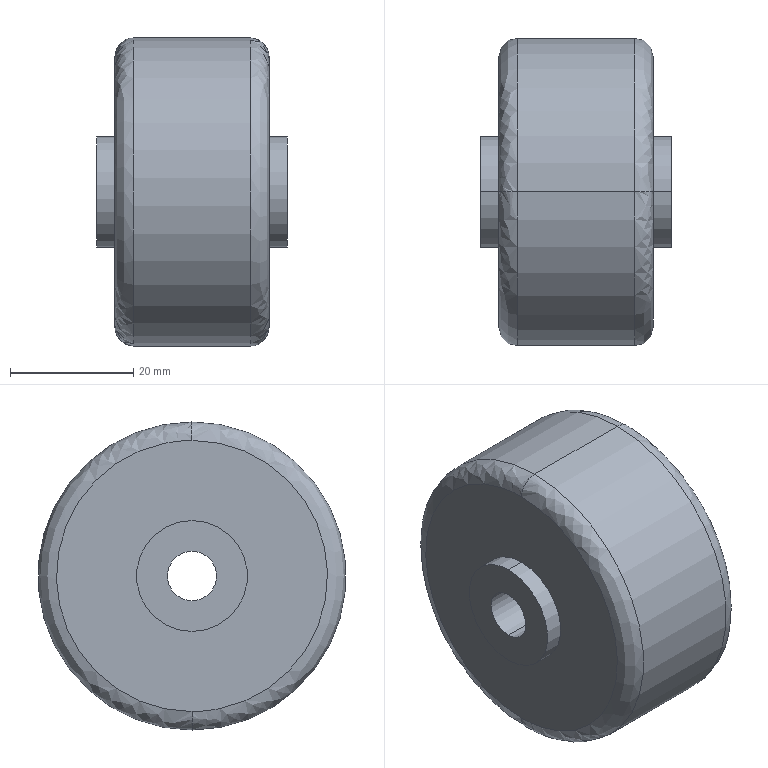Part | SolidWorks | features BaseBody 1 | 1 solid | 16 faces | box 31 x 50 x 50 mm | volume 48468 mm3 | cylinder 8 | spline 4 | plane 4 | commonest cylinder face diameters 18 x4 8 x2 50 x2
STEP:
#1=CARTESIAN_POINT('',(12.5,0.,-22.));
#2=VERTEX_POINT('',#1);
#3=CARTESIAN_POINT('',(12.5,0.,22.));
#4=VERTEX_POINT('',#3);
#5=CARTESIAN_POINT('',(12.5,0.,-22.));
#6=CARTESIAN_POINT('',(12.5,-44.,-22.));
#7=CARTESIAN_POINT('',(12.5,-44.,22.));
#8=CARTESIAN_POINT('',(12.5,0.,22.));
#9=(BOUNDED_CURVE()B_SPLINE_CURVE(3,(#5,#6,#7,#8),.UNSPECIFIED.,.F.,.F.)B_SPLINE_CURVE_WITH_KNOTS((4,4),(0.,0.5),.UNSPECIFIED.)CURVE()GEOMETRIC_REPRESENTATION_ITEM()RATIONAL_B_SPLINE_CURVE((1.,0.3333,0.3333,1.))REPRESENTATION_ITEM(''));
#10=EDGE_CURVE('',#2,#4,#9,.T.);
#11=ORIENTED_EDGE('',*,*,#10,.T.);
#12=CARTESIAN_POINT('',(9.5,0.,25.));
#13=VERTEX_POINT('',#12);
#14=CARTESIAN_POINT('',(9.5,0.,22.));
#15=DIRECTION('',(0.,-1.,0.));
#16=DIRECTION('',(0.,0.,1.));
#17=AXIS2_PLACEMENT_3D('',#14,#15,#16);
#18=CIRCLE('',#17,3.);
#19=EDGE_CURVE('',#4,#13,#18,.T.);
#20=ORIENTED_EDGE('',*,*,#19,.T.);
#21=CARTESIAN_POINT('',(9.5,0.,-25.));
#22=VERTEX_POINT('',#21);
#23=CARTESIAN_POINT('',(9.5,0.,0.));
#24=DIRECTION('',(-1.,0.,0.));
#25=DIRECTION('',(0.,0.,-1.));
#26=AXIS2_PLACEMENT_3D('',#23,#24,#25);
#27=CIRCLE('',#26,25.);
#28=EDGE_CURVE('',#22,#13,#27,.T.);
#29=ORIENTED_EDGE('',*,*,#28,.F.);
#30=CARTESIAN_POINT('',(9.5,0.,-22.));
#31=DIRECTION('',(0.,1.,0.));
#32=DIRECTION('',(0.,0.,-1.));
#33=AXIS2_PLACEMENT_3D('',#30,#31,#32);
#34=CIRCLE('',#33,3.);
#35=EDGE_CURVE('',#2,#22,#34,.T.);
#36=ORIENTED_EDGE('',*,*,#35,.F.);
#37=EDGE_LOOP('',(#11,#20,#29,#36));
#38=FACE_OUTER_BOUND('',#37,.T.);
#39=CARTESIAN_POINT('',(12.5,0.,22.));
#40=CARTESIAN_POINT('',(12.5,-44.,22.));
#41=CARTESIAN_POINT('',(12.5,-44.,-22.));
#42=CARTESIAN_POINT('',(12.5,0.,-22.));
#43=CARTESIAN_POINT('',(12.5,0.,23.757));
#44=CARTESIAN_POINT('',(12.5,-47.515,23.757));
#45=CARTESIAN_POINT('',(12.5,-47.515,-23.757));
#46=CARTESIAN_POINT('',(12.5,0.,-23.757));
#47=CARTESIAN_POINT('',(11.257,0.,25.));
#48=CARTESIAN_POINT('',(11.257,-50.,25.));
#49=CARTESIAN_POINT('',(11.257,-50.,-25.));
#50=CARTESIAN_POINT('',(11.257,0.,-25.));
#51=CARTESIAN_POINT('',(9.5,0.,25.));
#52=CARTESIAN_POINT('',(9.5,-50.,25.));
#53=CARTESIAN_POINT('',(9.5,-50.,-25.));
#54=CARTESIAN_POINT('',(9.5,0.,-25.));
#55=(BOUNDED_SURFACE()B_SPLINE_SURFACE(3,3,((#39,#40,#41,#42),(#43,#44,#45,#46),(#47,#48,#49,#50),(#51,#52,#53,#54)),.UNSPECIFIED.,.F.,.F.,.F.)B_SPLINE_SURFACE_WITH_KNOTS((4,4),(4,4),(0.,1.),(0.,1.),.UNSPECIFIED.)GEOMETRIC_REPRESENTATION_ITEM()RATIONAL_B_SPLINE_SURFACE(((1.,0.3333,0.3333,1.),(0.8047,0.2682,0.2682,0.8047),(0.8047,0.2682,0.2682,0.8047),(1.,0.3333,0.3333,1.)))REPRESENTATION_ITEM('')SURFACE());
#56=ADVANCED_FACE('',(#38),#55,.T.);
#57=CARTESIAN_POINT('',(-9.5,0.,25.));
#58=VERTEX_POINT('',#57);
#59=CARTESIAN_POINT('',(-9.5,0.,-25.));
#60=VERTEX_POINT('',#59);
#61=CARTESIAN_POINT('',(-9.5,0.,0.));
#62=DIRECTION('',(1.,0.,0.));
#63=DIRECTION('',(0.,0.,-1.));
#64=AXIS2_PLACEMENT_3D('',#61,#62,#63);
#65=CIRCLE('',#64,25.);
#66=EDGE_CURVE('',#58,#60,#65,.T.);
#67=ORIENTED_EDGE('',*,*,#66,.F.);
#68=CARTESIAN_POINT('',(-12.5,0.,22.));
#69=VERTEX_POINT('',#68);
#70=CARTESIAN_POINT('',(-9.5,0.,22.));
#71=DIRECTION('',(0.,-1.,0.));
#72=DIRECTION('',(0.,0.,1.));
#73=AXIS2_PLACEMENT_3D('',#70,#71,#72);
#74=CIRCLE('',#73,3.);
#75=EDGE_CURVE('',#58,#69,#74,.T.);
#76=ORIENTED_EDGE('',*,*,#75,.T.);
#77=CARTESIAN_POINT('',(-12.5,0.,-22.));
#78=VERTEX_POINT('',#77);
#79=CARTESIAN_POINT('',(-12.5,0.,22.));
#80=CARTESIAN_POINT('',(-12.5,-44.,22.));
#81=CARTESIAN_POINT('',(-12.5,-44.,-22.));
#82=CARTESIAN_POINT('',(-12.5,0.,-22.));
#83=(BOUNDED_CURVE()B_SPLINE_CURVE(3,(#79,#80,#81,#82),.UNSPECIFIED.,.F.,.T.)B_SPLINE_CURVE_WITH_KNOTS((4,4),(0.5,1.),.UNSPECIFIED.)CURVE()GEOMETRIC_REPRESENTATION_ITEM()RATIONAL_B_SPLINE_CURVE((1.,0.3333,0.3333,1.))REPRESENTATION_ITEM(''));
#84=EDGE_CURVE('',#69,#78,#83,.T.);
#85=ORIENTED_EDGE('',*,*,#84,.T.);
#86=CARTESIAN_POINT('',(-9.5,0.,-22.));
#87=DIRECTION('',(0.,1.,0.));
#88=DIRECTION('',(0.,0.,-1.));
#89=AXIS2_PLACEMENT_3D('',#86,#87,#88);
#90=CIRCLE('',#89,3.);
#91=EDGE_CURVE('',#60,#78,#90,.T.);
#92=ORIENTED_EDGE('',*,*,#91,.F.);
#93=EDGE_LOOP('',(#67,#76,#85,#92));
#94=FACE_OUTER_BOUND('',#93,.T.);
#95=CARTESIAN_POINT('',(-9.5,0.,25.));
#96=CARTESIAN_POINT('',(-9.5,-50.,25.));
#97=CARTESIAN_POINT('',(-9.5,-50.,-25.));
#98=CARTESIAN_POINT('',(-9.5,0.,-25.));
#99=CARTESIAN_POINT('',(-11.257,0.,25.));
#100=CARTESIAN_POINT('',(-11.257,-50.,25.));
#101=CARTESIAN_POINT('',(-11.257,-50.,-25.));
#102=CARTESIAN_POINT('',(-11.257,0.,-25.));
#103=CARTESIAN_POINT('',(-12.5,0.,23.757));
#104=CARTESIAN_POINT('',(-12.5,-47.515,23.757));
#105=CARTESIAN_POINT('',(-12.5,-47.515,-23.757));
#106=CARTESIAN_POINT('',(-12.5,0.,-23.757));
#107=CARTESIAN_POINT('',(-12.5,0.,22.));
#108=CARTESIAN_POINT('',(-12.5,-44.,22.));
#109=CARTESIAN_POINT('',(-12.5,-44.,-22.));
#110=CARTESIAN_POINT('',(-12.5,0.,-22.));
#111=(BOUNDED_SURFACE()B_SPLINE_SURFACE(3,3,((#95,#96,#97,#98),(#99,#100,#101,#102),(#103,#104,#105,#106),(#107,#108,#109,#110)),.UNSPECIFIED.,.F.,.F.,.F.)B_SPLINE_SURFACE_WITH_KNOTS((4,4),(4,4),(0.,1.),(0.,1.),.UNSPECIFIED.)GEOMETRIC_REPRESENTATION_ITEM()RATIONAL_B_SPLINE_SURFACE(((1.,0.3333,0.3333,1.),(0.8047,0.2682,0.2682,0.8047),(0.8047,0.2682,0.2682,0.8047),(1.,0.3333,0.3333,1.)))REPRESENTATION_ITEM('')SURFACE());
#112=ADVANCED_FACE('',(#94),#111,.T.);
#113=CARTESIAN_POINT('',(-9.5,0.,0.));
#114=DIRECTION('',(1.,0.,0.));
#115=DIRECTION('',(0.,0.,-1.));
#116=AXIS2_PLACEMENT_3D('',#113,#114,#115);
#117=CIRCLE('',#116,25.);
#118=EDGE_CURVE('',#60,#58,#117,.T.);
#119=ORIENTED_EDGE('',*,*,#118,.T.);
#120=CARTESIAN_POINT('',(15.5,0.,25.));
#121=DIRECTION('',(1.,0.,0.));
#122=VECTOR('',#121,1000.);
#123=LINE('',#120,#122);
#124=EDGE_CURVE('',#58,#13,#123,.T.);
#125=ORIENTED_EDGE('',*,*,#124,.T.);
#126=CARTESIAN_POINT('',(9.5,0.,0.));
#127=DIRECTION('',(-1.,0.,0.));
#128=DIRECTION('',(0.,0.,-1.));
#129=AXIS2_PLACEMENT_3D('',#126,#127,#128);
#130=CIRCLE('',#129,25.);
#131=EDGE_CURVE('',#13,#22,#130,.T.);
#132=ORIENTED_EDGE('',*,*,#131,.T.);
#133=CARTESIAN_POINT('',(15.5,0.,-25.));
#134=DIRECTION('',(1.,0.,0.));
#135=VECTOR('',#134,1000.);
#136=LINE('',#133,#135);
#137=EDGE_CURVE('',#60,#22,#136,.T.);
#138=ORIENTED_EDGE('',*,*,#137,.F.);
#139=EDGE_LOOP('',(#119,#125,#132,#138));
#140=FACE_OUTER_BOUND('',#139,.T.);
#141=CARTESIAN_POINT('',(15.5,0.,0.));
#142=DIRECTION('',(1.,0.,0.));
#143=DIRECTION('',(0.,0.,-1.));
#144=AXIS2_PLACEMENT_3D('',#141,#142,#143);
#145=CYLINDRICAL_SURFACE('',#144,25.);
#146=ADVANCED_FACE('',(#140),#145,.T.);
#147=CARTESIAN_POINT('',(12.5,0.,9.));
#148=VERTEX_POINT('',#147);
#149=CARTESIAN_POINT('',(12.5,0.,-9.));
#150=VERTEX_POINT('',#149);
#151=CARTESIAN_POINT('',(12.5,0.,0.));
#152=DIRECTION('',(-1.,0.,0.));
#153=DIRECTION('',(0.,0.,-1.));
#154=AXIS2_PLACEMENT_3D('',#151,#152,#153);
#155=CIRCLE('',#154,9.);
#156=EDGE_CURVE('',#148,#150,#155,.T.);
#157=ORIENTED_EDGE('',*,*,#156,.F.);
#158=CARTESIAN_POINT('',(15.5,0.,9.));
#159=VERTEX_POINT('',#158);
#160=CARTESIAN_POINT('',(15.5,0.,9.));
#161=DIRECTION('',(1.,0.,0.));
#162=VECTOR('',#161,1000.);
#163=LINE('',#160,#162);
#164=EDGE_CURVE('',#148,#159,#163,.T.);
#165=ORIENTED_EDGE('',*,*,#164,.T.);
#166=CARTESIAN_POINT('',(15.5,0.,-9.));
#167=VERTEX_POINT('',#166);
#168=CARTESIAN_POINT('',(15.5,0.,0.));
#169=DIRECTION('',(-1.,0.,0.));
#170=DIRECTION('',(0.,0.,-1.));
#171=AXIS2_PLACEMENT_3D('',#168,#169,#170);
#172=CIRCLE('',#171,9.);
#173=EDGE_CURVE('',#159,#167,#172,.T.);
#174=ORIENTED_EDGE('',*,*,#173,.T.);
#175=CARTESIAN_POINT('',(15.5,0.,-9.));
#176=DIRECTION('',(1.,0.,0.));
#177=VECTOR('',#176,1000.);
#178=LINE('',#175,#177);
#179=EDGE_CURVE('',#150,#167,#178,.T.);
#180=ORIENTED_EDGE('',*,*,#179,.F.);
#181=EDGE_LOOP('',(#157,#165,#174,#180));
#182=FACE_OUTER_BOUND('',#181,.T.);
#183=CARTESIAN_POINT('',(15.5,0.,0.));
#184=DIRECTION('',(1.,0.,0.));
#185=DIRECTION('',(0.,0.,-1.));
#186=AXIS2_PLACEMENT_3D('',#183,#184,#185);
#187=CYLINDRICAL_SURFACE('',#186,9.);
#188=ADVANCED_FACE('',(#182),#187,.T.);
#189=CARTESIAN_POINT('',(-15.5,0.,-9.));
#190=VERTEX_POINT('',#189);
#191=CARTESIAN_POINT('',(-15.5,0.,9.));
#192=VERTEX_POINT('',#191);
#193=CARTESIAN_POINT('',(-15.5,0.,0.));
#194=DIRECTION('',(1.,0.,0.));
#195=DIRECTION('',(0.,0.,-1.));
#196=AXIS2_PLACEMENT_3D('',#193,#194,#195);
#197=CIRCLE('',#196,9.);
#198=EDGE_CURVE('',#190,#192,#197,.T.);
#199=ORIENTED_EDGE('',*,*,#198,.T.);
#200=CARTESIAN_POINT('',(-12.5,0.,9.));
#201=VERTEX_POINT('',#200);
#202=CARTESIAN_POINT('',(15.5,0.,9.));
#203=DIRECTION('',(1.,0.,0.));
#204=VECTOR('',#203,1000.);
#205=LINE('',#202,#204);
#206=EDGE_CURVE('',#192,#201,#205,.T.);
#207=ORIENTED_EDGE('',*,*,#206,.T.);
#208=CARTESIAN_POINT('',(-12.5,0.,-9.));
#209=VERTEX_POINT('',#208);
#210=CARTESIAN_POINT('',(-12.5,0.,0.));
#211=DIRECTION('',(1.,0.,0.));
#212=DIRECTION('',(0.,0.,-1.));
#213=AXIS2_PLACEMENT_3D('',#210,#211,#212);
#214=CIRCLE('',#213,9.);
#215=EDGE_CURVE('',#209,#201,#214,.T.);
#216=ORIENTED_EDGE('',*,*,#215,.F.);
#217=CARTESIAN_POINT('',(15.5,0.,-9.));
#218=DIRECTION('',(1.,0.,0.));
#219=VECTOR('',#218,1000.);
#220=LINE('',#217,#219);
#221=EDGE_CURVE('',#190,#209,#220,.T.);
#222=ORIENTED_EDGE('',*,*,#221,.F.);
#223=EDGE_LOOP('',(#199,#207,#216,#222));
#224=FACE_OUTER_BOUND('',#223,.T.);
#225=CARTESIAN_POINT('',(15.5,0.,0.));
#226=DIRECTION('',(1.,0.,0.));
#227=DIRECTION('',(0.,0.,-1.));
#228=AXIS2_PLACEMENT_3D('',#225,#226,#227);
#229=CYLINDRICAL_SURFACE('',#228,9.);
#230=ADVANCED_FACE('',(#224),#229,.T.);
#231=CARTESIAN_POINT('',(-15.5,0.,4.));
#232=VERTEX_POINT('',#231);
#233=CARTESIAN_POINT('',(-15.5,0.,-4.));
#234=VERTEX_POINT('',#233);
#235=CARTESIAN_POINT('',(-15.5,0.,0.));
#236=DIRECTION('',(1.,0.,0.));
#237=DIRECTION('',(0.,0.,-1.));
#238=AXIS2_PLACEMENT_3D('',#235,#236,#237);
#239=CIRCLE('',#238,4.);
#240=EDGE_CURVE('',#232,#234,#239,.T.);
#241=ORIENTED_EDGE('',*,*,#240,.F.);
#242=CARTESIAN_POINT('',(15.5,0.,4.));
#243=VERTEX_POINT('',#242);
#244=CARTESIAN_POINT('',(15.5,0.,4.));
#245=DIRECTION('',(1.,0.,0.));
#246=VECTOR('',#245,1000.);
#247=LINE('',#244,#246);
#248=EDGE_CURVE('',#232,#243,#247,.T.);
#249=ORIENTED_EDGE('',*,*,#248,.T.);
#250=CARTESIAN_POINT('',(15.5,0.,-4.));
#251=VERTEX_POINT('',#250);
#252=CARTESIAN_POINT('',(15.5,0.,0.));
#253=DIRECTION('',(-1.,0.,0.));
#254=DIRECTION('',(0.,0.,-1.));
#255=AXIS2_PLACEMENT_3D('',#252,#253,#254);
#256=CIRCLE('',#255,4.);
#257=EDGE_CURVE('',#251,#243,#256,.T.);
#258=ORIENTED_EDGE('',*,*,#257,.F.);
#259=CARTESIAN_POINT('',(15.5,0.,-4.));
#260=DIRECTION('',(1.,0.,0.));
#261=VECTOR('',#260,1000.);
#262=LINE('',#259,#261);
#263=EDGE_CURVE('',#234,#251,#262,.T.);
#264=ORIENTED_EDGE('',*,*,#263,.F.);
#265=EDGE_LOOP('',(#241,#249,#258,#264));
#266=FACE_OUTER_BOUND('',#265,.T.);
#267=CARTESIAN_POINT('',(15.5,0.,0.));
#268=DIRECTION('',(1.,0.,0.));
#269=DIRECTION('',(0.,0.,-1.));
#270=AXIS2_PLACEMENT_3D('',#267,#268,#269);
#271=CYLINDRICAL_SURFACE('',#270,4.);
#272=ADVANCED_FACE('',(#266),#271,.F.);
#273=ORIENTED_EDGE('',*,*,#124,.F.);
#274=ORIENTED_EDGE('',*,*,#66,.T.);
#275=ORIENTED_EDGE('',*,*,#137,.T.);
#276=ORIENTED_EDGE('',*,*,#28,.T.);
#277=EDGE_LOOP('',(#273,#274,#275,#276));
#278=FACE_OUTER_BOUND('',#277,.T.);
#279=CARTESIAN_POINT('',(15.5,0.,0.));
#280=DIRECTION('',(1.,0.,0.));
#281=DIRECTION('',(0.,0.,-1.));
#282=AXIS2_PLACEMENT_3D('',#279,#280,#281);
#283=CYLINDRICAL_SURFACE('',#282,25.);
#284=ADVANCED_FACE('',(#278),#283,.T.);
#285=ORIENTED_EDGE('',*,*,#19,.F.);
#286=CARTESIAN_POINT('',(12.5,0.,22.));
#287=CARTESIAN_POINT('',(12.5,44.,22.));
#288=CARTESIAN_POINT('',(12.5,44.,-22.));
#289=CARTESIAN_POINT('',(12.5,0.,-22.));
#290=(BOUNDED_CURVE()B_SPLINE_CURVE(3,(#286,#287,#288,#289),.UNSPECIFIED.,.F.,.T.)B_SPLINE_CURVE_WITH_KNOTS((4,4),(0.5,1.),.UNSPECIFIED.)CURVE()GEOMETRIC_REPRESENTATION_ITEM()RATIONAL_B_SPLINE_CURVE((1.,0.3333,0.3333,1.))REPRESENTATION_ITEM(''));
#291=EDGE_CURVE('',#4,#2,#290,.T.);
#292=ORIENTED_EDGE('',*,*,#291,.T.);
#293=ORIENTED_EDGE('',*,*,#35,.T.);
#294=ORIENTED_EDGE('',*,*,#131,.F.);
#295=EDGE_LOOP('',(#285,#292,#293,#294));
#296=FACE_OUTER_BOUND('',#295,.T.);
#297=CARTESIAN_POINT('',(12.5,0.,-22.));
#298=CARTESIAN_POINT('',(12.5,44.,-22.));
#299=CARTESIAN_POINT('',(12.5,44.,22.));
#300=CARTESIAN_POINT('',(12.5,0.,22.));
#301=CARTESIAN_POINT('',(12.5,0.,-23.757));
#302=CARTESIAN_POINT('',(12.5,47.515,-23.757));
#303=CARTESIAN_POINT('',(12.5,47.515,23.757));
#304=CARTESIAN_POINT('',(12.5,0.,23.757));
#305=CARTESIAN_POINT('',(11.257,0.,-25.));
#306=CARTESIAN_POINT('',(11.257,50.,-25.));
#307=CARTESIAN_POINT('',(11.257,50.,25.));
#308=CARTESIAN_POINT('',(11.257,0.,25.));
#309=CARTESIAN_POINT('',(9.5,0.,-25.));
#310=CARTESIAN_POINT('',(9.5,50.,-25.));
#311=CARTESIAN_POINT('',(9.5,50.,25.));
#312=CARTESIAN_POINT('',(9.5,0.,25.));
#313=(BOUNDED_SURFACE()B_SPLINE_SURFACE(3,3,((#297,#298,#299,#300),(#301,#302,#303,#304),(#305,#306,#307,#308),(#309,#310,#311,#312)),.UNSPECIFIED.,.F.,.F.,.F.)B_SPLINE_SURFACE_WITH_KNOTS((4,4),(4,4),(0.,1.),(0.,1.),.UNSPECIFIED.)GEOMETRIC_REPRESENTATION_ITEM()RATIONAL_B_SPLINE_SURFACE(((1.,0.3333,0.3333,1.),(0.8047,0.2682,0.2682,0.8047),(0.8047,0.2682,0.2682,0.8047),(1.,0.3333,0.3333,1.)))REPRESENTATION_ITEM('')SURFACE());
#314=ADVANCED_FACE('',(#296),#313,.T.);
#315=ORIENTED_EDGE('',*,*,#75,.F.);
#316=ORIENTED_EDGE('',*,*,#118,.F.);
#317=ORIENTED_EDGE('',*,*,#91,.T.);
#318=CARTESIAN_POINT('',(-12.5,0.,-22.));
#319=CARTESIAN_POINT('',(-12.5,44.,-22.));
#320=CARTESIAN_POINT('',(-12.5,44.,22.));
#321=CARTESIAN_POINT('',(-12.5,0.,22.));
#322=(BOUNDED_CURVE()B_SPLINE_CURVE(3,(#318,#319,#320,#321),.UNSPECIFIED.,.F.,.T.)B_SPLINE_CURVE_WITH_KNOTS((4,4),(0.,0.5),.UNSPECIFIED.)CURVE()GEOMETRIC_REPRESENTATION_ITEM()RATIONAL_B_SPLINE_CURVE((1.,0.3333,0.3333,1.))REPRESENTATION_ITEM(''));
#323=EDGE_CURVE('',#78,#69,#322,.T.);
#324=ORIENTED_EDGE('',*,*,#323,.T.);
#325=EDGE_LOOP('',(#315,#316,#317,#324));
#326=FACE_OUTER_BOUND('',#325,.T.);
#327=CARTESIAN_POINT('',(-9.5,0.,-25.));
#328=CARTESIAN_POINT('',(-9.5,50.,-25.));
#329=CARTESIAN_POINT('',(-9.5,50.,25.));
#330=CARTESIAN_POINT('',(-9.5,0.,25.));
#331=CARTESIAN_POINT('',(-11.257,0.,-25.));
#332=CARTESIAN_POINT('',(-11.257,50.,-25.));
#333=CARTESIAN_POINT('',(-11.257,50.,25.));
#334=CARTESIAN_POINT('',(-11.257,0.,25.));
#335=CARTESIAN_POINT('',(-12.5,0.,-23.757));
#336=CARTESIAN_POINT('',(-12.5,47.515,-23.757));
#337=CARTESIAN_POINT('',(-12.5,47.515,23.757));
#338=CARTESIAN_POINT('',(-12.5,0.,23.757));
#339=CARTESIAN_POINT('',(-12.5,0.,-22.));
#340=CARTESIAN_POINT('',(-12.5,44.,-22.));
#341=CARTESIAN_POINT('',(-12.5,44.,22.));
#342=CARTESIAN_POINT('',(-12.5,0.,22.));
#343=(BOUNDED_SURFACE()B_SPLINE_SURFACE(3,3,((#327,#328,#329,#330),(#331,#332,#333,#334),(#335,#336,#337,#338),(#339,#340,#341,#342)),.UNSPECIFIED.,.F.,.F.,.F.)B_SPLINE_SURFACE_WITH_KNOTS((4,4),(4,4),(0.,1.),(0.,1.),.UNSPECIFIED.)GEOMETRIC_REPRESENTATION_ITEM()RATIONAL_B_SPLINE_SURFACE(((1.,0.3333,0.3333,1.),(0.8047,0.2682,0.2682,0.8047),(0.8047,0.2682,0.2682,0.8047),(1.,0.3333,0.3333,1.)))REPRESENTATION_ITEM('')SURFACE());
#344=ADVANCED_FACE('',(#326),#343,.T.);
#345=CARTESIAN_POINT('',(12.5,0.,0.));
#346=DIRECTION('',(-1.,0.,0.));
#347=DIRECTION('',(0.,0.,-1.));
#348=AXIS2_PLACEMENT_3D('',#345,#346,#347);
#349=CIRCLE('',#348,9.);
#350=EDGE_CURVE('',#150,#148,#349,.T.);
#351=ORIENTED_EDGE('',*,*,#350,.T.);
#352=ORIENTED_EDGE('',*,*,#156,.T.);
#353=EDGE_LOOP('',(#351,#352));
#354=FACE_BOUND('',#353,.T.);
#355=ORIENTED_EDGE('',*,*,#10,.F.);
#356=ORIENTED_EDGE('',*,*,#291,.F.);
#357=EDGE_LOOP('',(#355,#356));
#358=FACE_OUTER_BOUND('',#357,.T.);
#359=CARTESIAN_POINT('',(12.5,9.,0.));
#360=DIRECTION('',(1.,0.,0.));
#361=DIRECTION('',(0.,0.,-1.));
#362=AXIS2_PLACEMENT_3D('',#359,#360,#361);
#363=PLANE('',#362);
#364=ADVANCED_FACE('',(#354,#358),#363,.T.);
#365=ORIENTED_EDGE('',*,*,#323,.F.);
#366=ORIENTED_EDGE('',*,*,#84,.F.);
#367=EDGE_LOOP('',(#365,#366));
#368=FACE_OUTER_BOUND('',#367,.T.);
#369=ORIENTED_EDGE('',*,*,#215,.T.);
#370=CARTESIAN_POINT('',(-12.5,0.,0.));
#371=DIRECTION('',(1.,0.,0.));
#372=DIRECTION('',(0.,0.,-1.));
#373=AXIS2_PLACEMENT_3D('',#370,#371,#372);
#374=CIRCLE('',#373,9.);
#375=EDGE_CURVE('',#201,#209,#374,.T.);
#376=ORIENTED_EDGE('',*,*,#375,.T.);
#377=EDGE_LOOP('',(#369,#376));
#378=FACE_BOUND('',#377,.T.);
#379=CARTESIAN_POINT('',(-12.5,22.,0.));
#380=DIRECTION('',(-1.,0.,0.));
#381=DIRECTION('',(0.,0.,1.));
#382=AXIS2_PLACEMENT_3D('',#379,#380,#381);
#383=PLANE('',#382);
#384=ADVANCED_FACE('',(#368,#378),#383,.T.);
#385=ORIENTED_EDGE('',*,*,#164,.F.);
#386=ORIENTED_EDGE('',*,*,#350,.F.);
#387=ORIENTED_EDGE('',*,*,#179,.T.);
#388=CARTESIAN_POINT('',(15.5,0.,0.));
#389=DIRECTION('',(-1.,0.,0.));
#390=DIRECTION('',(0.,0.,-1.));
#391=AXIS2_PLACEMENT_3D('',#388,#389,#390);
#392=CIRCLE('',#391,9.);
#393=EDGE_CURVE('',#167,#159,#392,.T.);
#394=ORIENTED_EDGE('',*,*,#393,.T.);
#395=EDGE_LOOP('',(#385,#386,#387,#394));
#396=FACE_OUTER_BOUND('',#395,.T.);
#397=CARTESIAN_POINT('',(15.5,0.,0.));
#398=DIRECTION('',(1.,0.,0.));
#399=DIRECTION('',(0.,0.,-1.));
#400=AXIS2_PLACEMENT_3D('',#397,#398,#399);
#401=CYLINDRICAL_SURFACE('',#400,9.);
#402=ADVANCED_FACE('',(#396),#401,.T.);
#403=ORIENTED_EDGE('',*,*,#206,.F.);
#404=CARTESIAN_POINT('',(-15.5,0.,0.));
#405=DIRECTION('',(1.,0.,0.));
#406=DIRECTION('',(0.,0.,-1.));
#407=AXIS2_PLACEMENT_3D('',#404,#405,#406);
#408=CIRCLE('',#407,9.);
#409=EDGE_CURVE('',#192,#190,#408,.T.);
#410=ORIENTED_EDGE('',*,*,#409,.T.);
#411=ORIENTED_EDGE('',*,*,#221,.T.);
#412=ORIENTED_EDGE('',*,*,#375,.F.);
#413=EDGE_LOOP('',(#403,#410,#411,#412));
#414=FACE_OUTER_BOUND('',#413,.T.);
#415=CARTESIAN_POINT('',(15.5,0.,0.));
#416=DIRECTION('',(1.,0.,0.));
#417=DIRECTION('',(0.,0.,-1.));
#418=AXIS2_PLACEMENT_3D('',#415,#416,#417);
#419=CYLINDRICAL_SURFACE('',#418,9.);
#420=ADVANCED_FACE('',(#414),#419,.T.);
#421=ORIENTED_EDGE('',*,*,#257,.T.);
#422=CARTESIAN_POINT('',(15.5,0.,0.));
#423=DIRECTION('',(-1.,0.,0.));
#424=DIRECTION('',(0.,0.,-1.));
#425=AXIS2_PLACEMENT_3D('',#422,#423,#424);
#426=CIRCLE('',#425,4.);
#427=EDGE_CURVE('',#243,#251,#426,.T.);
#428=ORIENTED_EDGE('',*,*,#427,.T.);
#429=EDGE_LOOP('',(#421,#428));
#430=FACE_BOUND('',#429,.T.);
#431=ORIENTED_EDGE('',*,*,#393,.F.);
#432=ORIENTED_EDGE('',*,*,#173,.F.);
#433=EDGE_LOOP('',(#431,#432));
#434=FACE_OUTER_BOUND('',#433,.T.);
#435=CARTESIAN_POINT('',(15.5,4.,0.));
#436=DIRECTION('',(1.,0.,0.));
#437=DIRECTION('',(0.,0.,-1.));
#438=AXIS2_PLACEMENT_3D('',#435,#436,#437);
#439=PLANE('',#438);
#440=ADVANCED_FACE('',(#430,#434),#439,.T.);
#441=ORIENTED_EDGE('',*,*,#198,.F.);
#442=ORIENTED_EDGE('',*,*,#409,.F.);
#443=EDGE_LOOP('',(#441,#442));
#444=FACE_OUTER_BOUND('',#443,.T.);
#445=CARTESIAN_POINT('',(-15.5,0.,0.));
#446=DIRECTION('',(1.,0.,0.));
#447=DIRECTION('',(0.,0.,-1.));
#448=AXIS2_PLACEMENT_3D('',#445,#446,#447);
#449=CIRCLE('',#448,4.);
#450=EDGE_CURVE('',#234,#232,#449,.T.);
#451=ORIENTED_EDGE('',*,*,#450,.T.);
#452=ORIENTED_EDGE('',*,*,#240,.T.);
#453=EDGE_LOOP('',(#451,#452));
#454=FACE_BOUND('',#453,.T.);
#455=CARTESIAN_POINT('',(-15.5,9.,0.));
#456=DIRECTION('',(-1.,0.,0.));
#457=DIRECTION('',(0.,0.,1.));
#458=AXIS2_PLACEMENT_3D('',#455,#456,#457);
#459=PLANE('',#458);
#460=ADVANCED_FACE('',(#444,#454),#459,.T.);
#461=ORIENTED_EDGE('',*,*,#248,.F.);
#462=ORIENTED_EDGE('',*,*,#450,.F.);
#463=ORIENTED_EDGE('',*,*,#263,.T.);
#464=ORIENTED_EDGE('',*,*,#427,.F.);
#465=EDGE_LOOP('',(#461,#462,#463,#464));
#466=FACE_OUTER_BOUND('',#465,.T.);
#467=CARTESIAN_POINT('',(15.5,0.,0.));
#468=DIRECTION('',(1.,0.,0.));
#469=DIRECTION('',(0.,0.,-1.));
#470=AXIS2_PLACEMENT_3D('',#467,#468,#469);
#471=CYLINDRICAL_SURFACE('',#470,4.);
#472=ADVANCED_FACE('',(#466),#471,.F.);
#473=CLOSED_SHELL('',(#56,#112,#146,#188,#230,#272,#284,#314,#344,#364,#384,#402,#420,#440,#460,#472));
#474=MANIFOLD_SOLID_BREP('',#473);
#475=CARTESIAN_POINT('',(0.,0.,0.));
#476=DIRECTION('',(0.,0.,1.));
#477=DIRECTION('',(1.,0.,0.));
#478=AXIS2_PLACEMENT_3D('',#475,#476,#477);
#479=(LENGTH_UNIT()NAMED_UNIT(*)SI_UNIT(.MILLI.,.METRE.));
#480=UNCERTAINTY_MEASURE_WITH_UNIT(LENGTH_MEASURE(0.00001),#479,'','');
#481=(NAMED_UNIT(*)PLANE_ANGLE_UNIT()SI_UNIT($,.RADIAN.));
#482=(NAMED_UNIT(*)SI_UNIT($,.STERADIAN.)SOLID_ANGLE_UNIT());
#483=(GEOMETRIC_REPRESENTATION_CONTEXT(3)GLOBAL_UNCERTAINTY_ASSIGNED_CONTEXT((#480))GLOBAL_UNIT_ASSIGNED_CONTEXT((#479,#481,#482))REPRESENTATION_CONTEXT('',''));
#484=ADVANCED_BREP_SHAPE_REPRESENTATION('',(#474,#478),#483);